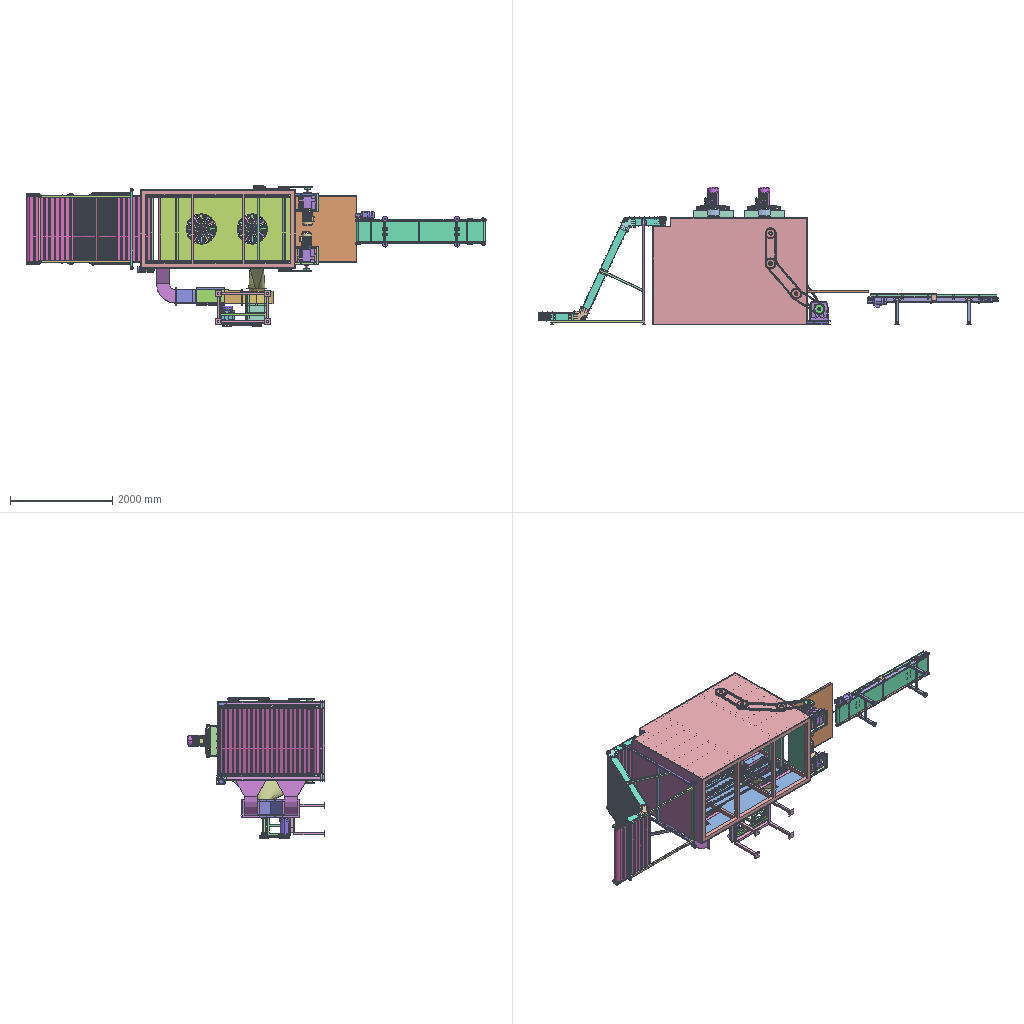Assembly | STEP file | 148 different items | 1898 placed | box 9018 x 2697 x 2745 mm
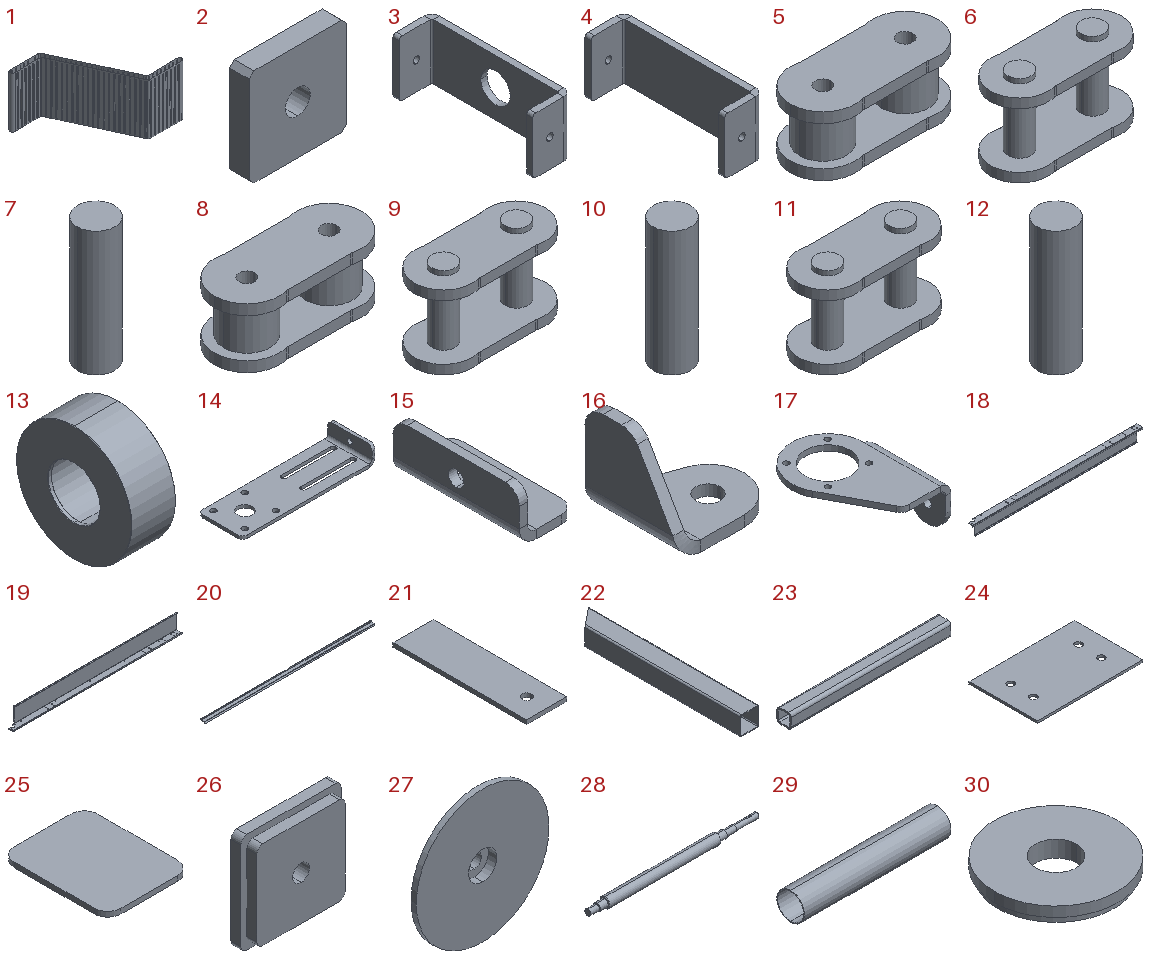Parts list (item | name | quantity | parent item | size | volume):
1 | Belt1-5^Produce dryer-Z conveyor | x1 | in Produce dryer-Z conveyor | 2487 x 2048 x 1290 mm | 28033863 mm3
2 | Bich chan tang chinh | x4 | in Produce dryer-Main support leg assembly | 40 x 8 x 40 mm | 12082 mm3
3 | Cang dai | x2 | in Produce dryer-Belt tensioner assembly | 25 x 90 x 36 mm | 17378 mm3
4 | Cang dai 2 | x2 | in Produce dryer-Belt tensioner assembly | 25 x 90 x 36 mm | 18513 mm3
5 | Chain 2-20A link 1 | x33 | in 链条2总成-00 | 56.75 x 25 x 23 mm | 16394 mm3
6 | Chain 2-20A link 2 | x33 | in 链条2总成-00 | 56.75 x 25 x 36 mm | 14459 mm3
7 | Chain 2-20A path | x1 | in 链条2总成-00 | 3 x 3 x 10 mm | 70.686 mm3
8 | Chain 3-20A link 1 | x56 | in 链条3总成-00 | 56.75 x 25 x 23 mm | 16394 mm3
9 | Chain 3-20A link 2 | x56 | in 链条3总成-00 | 56.75 x 25 x 36 mm | 14459 mm3
10 | Chain 3-20A path | x2 | in 链条3总成-00 | 3 x 3 x 10 mm | 70.686 mm3
11 | Chain 4-20A link 2 | x30 | in 链条4总成-00 | 56.75 x 25 x 36 mm | 14459 mm3
12 | Chain 4-20A path | x1 | in 链条4总成-00 | 3 x 3 x 10 mm | 70.686 mm3
13 | Con lan ty | x12 | in Roller assembly | 23 x 60 x 60 mm | 48906 mm3
14 | Flat conveyor mechanism-CN2500x400-101-101 | x2 | in 平输送机构-CN2500x400-101-100 | 270 x 90 x 36 mm | 137966 mm3
15 | Flat conveyor mechanism-CN2500x400-101-102 | x2 | in 平输送机构-CN2500x400-101-100 | 40 x 90 x 36 mm | 33488 mm3
16 | Flat conveyor mechanism-CN2500x400-102-101 | x1 | in Flat conveyor mechanism-CN2500x400-102-100 | 56 x 52 x 51 mm | 22223 mm3
17 | Flat conveyor mechanism-CN2500x400-102-102 | x1 | in Flat conveyor mechanism-CN2500x400-102-100 | 92 x 125 x 49 mm | 51756 mm3
18 | Flat conveyor mechanism-CN2500x400-103-101a | x1 | in Flat conveyor mechanism-assembly 2 | 2460 x 93 x 223 mm | 2426362 mm3
19 | Flat conveyor mechanism-CN2500x400-103-101b | x1 | in Flat conveyor mechanism-assembly 2 | 2460 x 100 x 223 mm | 2477714 mm3
20 | Flat conveyor mechanism-CN2500x400-104-101_DefaultSM-FLAT-PATTERN | x2 | in Flat conveyor mechanism-CN2500x400-104a-100, Flat conveyor mechanism-CN2500x400-104b-100 | 2450 x 58.268 x 35.821 mm | 594137 mm3
21 | Flat conveyor mechanism-CN2500x400-104-102 | x10 | in Flat conveyor mechanism-CN2500x400-104a-100, Flat conveyor mechanism-CN2500x400-104b-100 | 30 x 100 x 3 mm | 8885 mm3
22 | Flat conveyor mechanism-CN2500x400-105-101_Default<As machined> | x4 | in Flat conveyor mechanism-CN2500x400-105-100 | 50 x 450 x 50 mm | 160691 mm3
23 | Flat conveyor mechanism-CN2500x400-105-102_Default<As machined> | x2 | in Flat conveyor mechanism-CN2500x400-105-100 | 452 x 40 x 40 mm | 241728 mm3
24 | Flat conveyor mechanism-CN2500x400-105-103 | x4 | in Flat conveyor mechanism-CN2500x400-105-100 | 140 x 90 x 3 mm | 37037 mm3
25 | Flat conveyor mechanism-CN2500x400-105-104 | x4 | in Flat conveyor mechanism-CN2500x400-105-100 | 50 x 64 x 3 mm | 9435 mm3
26 | Flat conveyor mechanism-CN2500x400-105-105 | x4 | in Flat conveyor mechanism-CN2500x400-105-100 | 50 x 10 x 50 mm | 21535 mm3
27 | Flat conveyor mechanism-CN2500x400-105-106 | x4 | in 27 | 100 x 20 x 100 mm | 96687 mm3
28 | Flat conveyor mechanism-CN2500x400-107-101 | x1 | in Flat conveyor mechanism-CN2500x400-107-100 | 595.6 x 35 x 35 mm | 445688 mm3
29 | Flat conveyor mechanism-CN2500x400-107-102 | x2 | in Flat conveyor mechanism-CN2500x400-107-100, Flat conveyor mechanism-CN2500x400-108-100 | 400 x 75 x 75 mm | 183469 mm3
30 | Flat conveyor mechanism-CN2500x400-107-103 | x4 | in Flat conveyor mechanism-CN2500x400-107-100, Flat conveyor mechanism-CN2500x400-108-100 | 75 x 75 x 10 mm | 37435 mm3
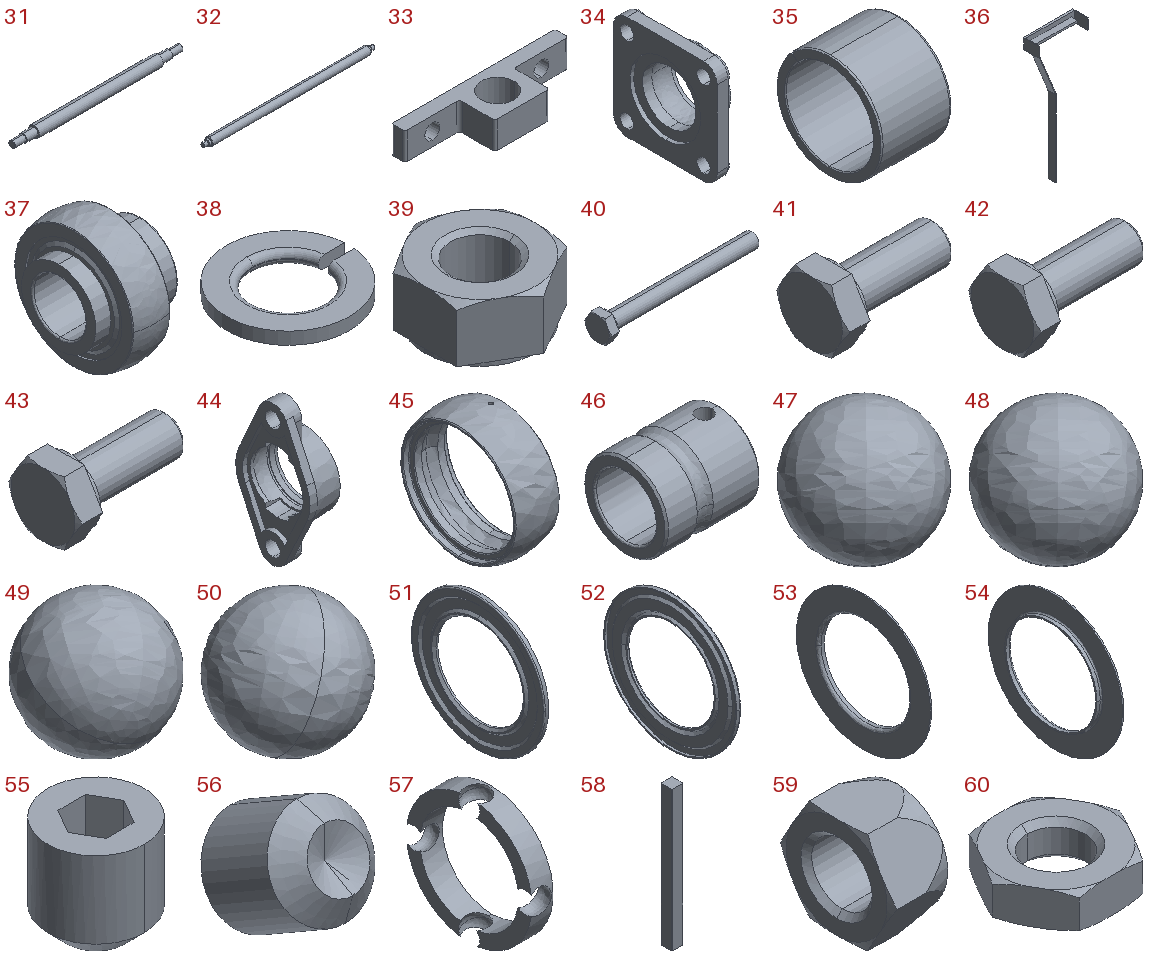31 | Flat conveyor mechanism-CN2500x400-108-101 | x1 | in Flat conveyor mechanism-CN2500x400-108-100 | 532 x 35 x 35 mm | 433255 mm3
32 | Flat conveyor mechanism-CN2500x400-111-101 | x3 | in Flat conveyor mechanism-CN2500x400-111-100 | 431 x 20 x 20 mm | 128796 mm3
33 | Flat conveyor mechanism-CN2500x400-111-102 | x6 | in Flat conveyor mechanism-CN2500x400-111-100 | 60 x 18 x 10 mm | 4223 mm3
34 | Flat conveyor mechanism-FY 504 U_VA228_fyva_Default | x2 | in Flat conveyor mechanism-FY 20 TF_VA228_Default | 29.5 x 86 x 86 mm | 59887 mm3
35 | Flat conveyor mechanism-PCM 101208 E.stp | x6 | in Flat conveyor mechanism-CN2500x400-111-100 | 8 x 12 x 12 mm | 274.832 mm3
36 | Flat conveyor mechanism-Part11 | x1 | in Flat conveyor mechanism-assembly 2 | 476 x 150 x 1294 mm | 1809742 mm3
37 | Flat conveyor mechanism-YAR 204-2FW_VA228_Default | x2 | in Flat conveyor mechanism-FY 20 TF_VA228_Default | 31 x 47 x 47 mm | 24116 mm3
38 | Flat conveyor mechanism-din_128_a12 | x12 | in 平输送机构-CN2500x400-101-100 | 21.067 x 21.1 x 2.1 mm | 456.756 mm3
39 | Flat conveyor mechanism-hex nut style 1 gradeab_din_Hexagon Nut ISO 4032 - M10 - W - N_Default | x4 | in 27 | 16 x 18.475 x 8.4 mm | 1357 mm3
40 | Flat conveyor mechanism-hex screw gradeab_din_DIN EN 24017 - M10 x 100-N_Default | x6 | in 27, 平输送机构-CN2500x400-101-100 | 106.4 x 18.475 x 16 mm | 9247 mm3
41 | Flat conveyor mechanism-hex screw gradeab_din_DIN EN 24017 - M10 x 25-N_Default | x2 | in Flat conveyor mechanism-assembly 2 | 31.4 x 18.475 x 16 mm | 3356 mm3
42 | Flat conveyor mechanism-hex screw gradeab_din_DIN EN 24017 - M6 x 16-N_Default | x16 | in Flat conveyor mechanism-assembly 2 | 20 x 11.547 x 10 mm | 791.21 mm3
43 | Flat conveyor mechanism-hex screw gradeab_din_DIN EN 24017 - M8 x 20-N_Default | x18 | in Flat conveyor mechanism-CN2500x400-102-100, Flat conveyor mechanism-assembly 2 | 25.3 x 15.011 x 13 mm | 1766 mm3
44 | Flat conveyor mechanism-inafag_ucfl204_62o9y6gnj3059x015y4y3bh4_01 | x2 | in Flat conveyor mechanism-inafag_ucfl204_62o9y6gnj3059x015y4y3bh4 | - | -
45 | Flat conveyor mechanism-inafag_ucfl204_62o9y6gnj3059x015y4y3bh4_02 | x2 | in Flat conveyor mechanism-inafag_ucfl204_62o9y6gnj3059x015y4y3bh4 | 17 x 47.603 x 47 mm | 6473 mm3
46 | Flat conveyor mechanism-inafag_ucfl204_62o9y6gnj3059x015y4y3bh4_03 | x2 | in Flat conveyor mechanism-inafag_ucfl204_62o9y6gnj3059x015y4y3bh4 | 31 x 27.56 x 27.56 mm | 8243 mm3
47 | Flat conveyor mechanism-inafag_ucfl204_62o9y6gnj3059x015y4y3bh4_04 | x2 | in Flat conveyor mechanism-inafag_ucfl204_62o9y6gnj3059x015y4y3bh4 | 7.94 x 7.94 x 7.94 mm | 262.089 mm3
48 | Flat conveyor mechanism-inafag_ucfl204_62o9y6gnj3059x015y4y3bh4_05 | x2 | in Flat conveyor mechanism-inafag_ucfl204_62o9y6gnj3059x015y4y3bh4 | 7.94 x 7.94 x 7.94 mm | 262.089 mm3
49 | Flat conveyor mechanism-inafag_ucfl204_62o9y6gnj3059x015y4y3bh4_06 | x2 | in Flat conveyor mechanism-inafag_ucfl204_62o9y6gnj3059x015y4y3bh4 | 7.94 x 7.94 x 7.94 mm | 262.089 mm3
50 | Flat conveyor mechanism-inafag_ucfl204_62o9y6gnj3059x015y4y3bh4_07 | x2 | in Flat conveyor mechanism-inafag_ucfl204_62o9y6gnj3059x015y4y3bh4 | 7.94 x 7.94 x 7.94 mm | 262.089 mm3
51 | Flat conveyor mechanism-inafag_ucfl204_62o9y6gnj3059x015y4y3bh4_08 | x2 | in Flat conveyor mechanism-inafag_ucfl204_62o9y6gnj3059x015y4y3bh4 | 1.397 x 42 x 42 mm | 599.425 mm3
52 | Flat conveyor mechanism-inafag_ucfl204_62o9y6gnj3059x015y4y3bh4_09 | x2 | in Flat conveyor mechanism-inafag_ucfl204_62o9y6gnj3059x015y4y3bh4 | 1.397 x 42 x 42 mm | 599.533 mm3
53 | Flat conveyor mechanism-inafag_ucfl204_62o9y6gnj3059x015y4y3bh4_10 | x2 | in Flat conveyor mechanism-inafag_ucfl204_62o9y6gnj3059x015y4y3bh4 | 1.812 x 41.16 x 41.16 mm | 343.087 mm3
54 | Flat conveyor mechanism-inafag_ucfl204_62o9y6gnj3059x015y4y3bh4_11 | x2 | in Flat conveyor mechanism-inafag_ucfl204_62o9y6gnj3059x015y4y3bh4 | 1.812 x 41.16 x 41.16 mm | 343.35 mm3
55 | Flat conveyor mechanism-inafag_ucfl204_62o9y6gnj3059x015y4y3bh4_12 | x2 | in Flat conveyor mechanism-inafag_ucfl204_62o9y6gnj3059x015y4y3bh4 | 6 x 6 x 6 mm | 135.214 mm3
56 | Flat conveyor mechanism-inafag_ucfl204_62o9y6gnj3059x015y4y3bh4_13 | x2 | in Flat conveyor mechanism-inafag_ucfl204_62o9y6gnj3059x015y4y3bh4 | 6 x 7.571 x 7.571 mm | 135.214 mm3
57 | Flat conveyor mechanism-inafag_ucfl204_62o9y6gnj3059x015y4y3bh4_14 | x2 | in Flat conveyor mechanism-inafag_ucfl204_62o9y6gnj3059x015y4y3bh4 | - | 2155 mm3
58 | Flat conveyor mechanism-key 6x6x70 | x1 | in Flat conveyor mechanism-assembly 2 | 6 x 6 x 75 mm | 2686 mm3
59 | Flat conveyor mechanism-nut_gb_t_6185_1_m6 | x16 | in Flat conveyor mechanism-assembly 2 | 6 x 11.547 x 10 mm | 336.581 mm3
60 | Flat conveyor mechanism-nut_iso_4035_-_d_m10_-_05 | x32 | in 平输送机构-CN2500x400-101-100 | 18.475 x 16 x 5 mm | 809.954 mm3
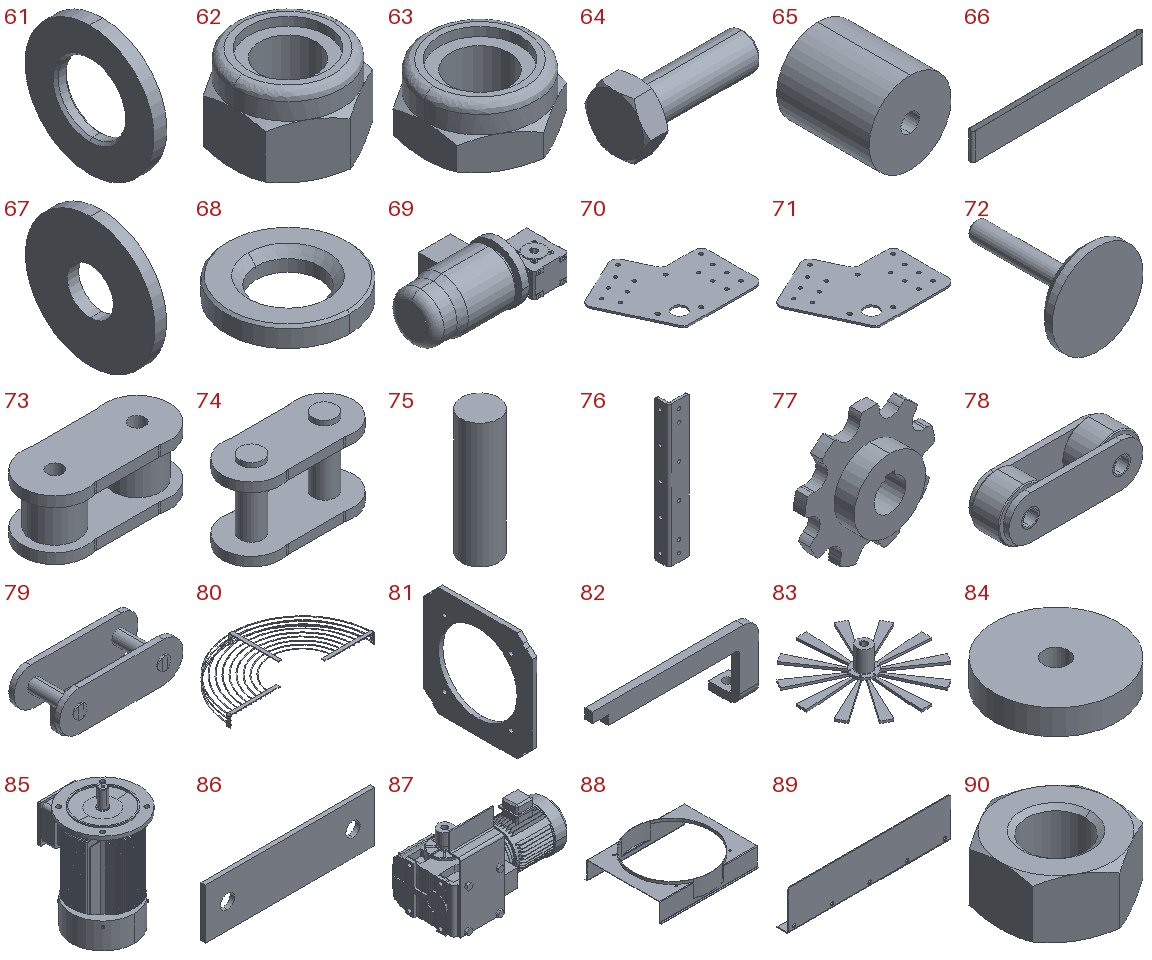61 | Flat conveyor mechanism-plain washer hardened grade a_din_Washer DIN 125 - A 10.5 - 300HV_Default | x4 | in Flat conveyor mechanism-assembly 2 | 2 x 20 x 20 mm | 449.726 mm3
62 | Flat conveyor mechanism-prevailing torque nut style 1 insert_din_DIN EN ISO 7040 - M8 - N_Default | x16 | in Flat conveyor mechanism-assembly 2 | 13 x 15.011 x 9.5 mm | 952.721 mm3
63 | Flat conveyor mechanism-prevailing torque nut thin insert_din_DIN EN ISO 10511 - M10 - N_Default | x2 | in Flat conveyor mechanism-assembly 2 | 16 x 18.475 x 8.56 mm | 1235 mm3
64 | Flat conveyor mechanism-screw_gb_t_6563_m10x30 | x20 | in 平输送机构-CN2500x400-101-100 | 36.4 x 18.475 x 16 mm | 3756 mm3
65 | Flat conveyor mechanism-silenbloc 40x45xm8 | x1 | in Flat conveyor mechanism-CN2500x400-102-100 | 40 x 45 x 40 mm | 54907 mm3
66 | Flat conveyor mechanism-strip | x1 | in Flat conveyor mechanism-assembly 2 | 2534 x 103.36 x 400 mm | 5769946 mm3
67 | Flat conveyor mechanism-washer_gb_t_96_1_6 | x12 | in Flat conveyor mechanism-assembly 2 | 1.6 x 18 x 18 mm | 355.679 mm3
68 | Flat conveyor mechanism-washer_iso_7416-12 | x40 | in 平输送机构-CN2500x400-101-100 | 25 x 25 x 4 mm | 1366 mm3
69 | Flat conveyor mechanism-worm gear reducer_mu40-base-10-b3 | x1 | in Flat conveyor mechanism-assembly 2 | 361 x 200 x 160 mm | 5383182 mm3
70 | Ga bi suong | x2 | in Produce dryer-Belt tensioner corner assembly | 306.397 x 266.767 x 5 mm | 273503 mm3
71 | Ga bi suong 2 | x2 | in Produce dryer-Corner belt tensioner assembly 2 | 306.397 x 266.767 x 5 mm | 273503 mm3
72 | Main support leg M12 for conveyor | x4 | in Produce dryer-Main support leg assembly | 60 x 80 x 60 mm | 33948 mm3
73 | Motor output chain-06B link 1 | x24 | in 电机输出链条-00 | 56.75 x 25 x 23 mm | 16394 mm3
74 | Motor output chain-06B link 2 | x24 | in 电机输出链条-00 | 56.75 x 25 x 36 mm | 14459 mm3
75 | Motor output chain-motor drive chain path 1 | x1 | in 电机输出链条-00 | 3 x 3 x 10 mm | 70.686 mm3
76 | Part 1 cang dai | x4 | in Produce dryer-Belt tensioner assembly | 36 x 25 x 250 mm | 54427 mm3
77 | Produce dryer 9-tooth 40 bore with keyway total width 40 C216AL sprocket | x20 | in Produce dryer single mesh belt assembly, Produce dryer single mesh belt assembly C | 163.79 x 40 x 161.93 mm | 358621 mm3
78 | Produce dryer C216AL inner link | x470 | in Produce dryer single mesh belt assembly, Produce dryer single mesh belt assembly C | - | -
79 | Produce dryer C216AL outer link | x470 | in Produce dryer single mesh belt assembly, Produce dryer single mesh belt assembly C | - | -
80 | Produce dryer HY-40-M-021 | x4 | in Produce dryer HY-40-M-700 | 645 x 322.5 x 50 mm | 90254 mm3
81 | Produce dryer HY-40-M-701 | x2 | in Produce dryer HY-40-M-710 | 10 x 250 x 250 mm | 341607 mm3
82 | Produce dryer HY-40-M-702 | x8 | in Produce dryer HY-40-M-710 | 215 x 40 x 90 mm | 72091 mm3
83 | Produce dryer HY-40-M-809 | x2 | in Produce dryer HY-40-M-700 | 550 x 550 x 113 mm | 1036820 mm3
84 | Produce dryer HY-40-M-bushing clamp plate | x2 | in Produce dryer HY-40-M-700 | 49 x 49 x 10 mm | 18072 mm3
85 | Produce dryer YE3-100L-4-B5_YE4-100L-2 | x2 | in Produce dryer HY-40-M-700 | 250 x 295 x 435 mm | 12374001 mm3
86 | Produce dryer bearing housing pad plate | x10 | in Produce dryer mesh belt assembly Type A, Produce dryer mesh belt assembly Type B, Produce dryer mesh belt assembly Type C | 185 x 5 x 55 mm | 48988 mm3
87 | Produce dryer conveyor belt NSNS47 reducer_NS 67 | x1 | in Produce dryer-Z conveyor | 331.6 x 173.674 x 227.5 mm | 3816631 mm3
88 | Produce dryer cooling section-HY-40-M-601 | x2 | in Produce dryer cooling section-HY-40-M-cover assembly | 786 x 630 x 168 mm | 1349163 mm3
89 | Produce dryer cooling section-HY-40-M-602 | x4 | in Produce dryer cooling section-HY-40-M-cover assembly | 584 x 40 x 142 mm | 308453 mm3
90 | Produce dryer cooling section-hex nut style 1_am_B18.2.4.1M - Hex nut, Style 1, M10 x 1.5 | x8 | in Produce dryer cooling section-HY-40-M-cover assembly | 16 x 18.475 x 8.4 mm | 1365 mm3
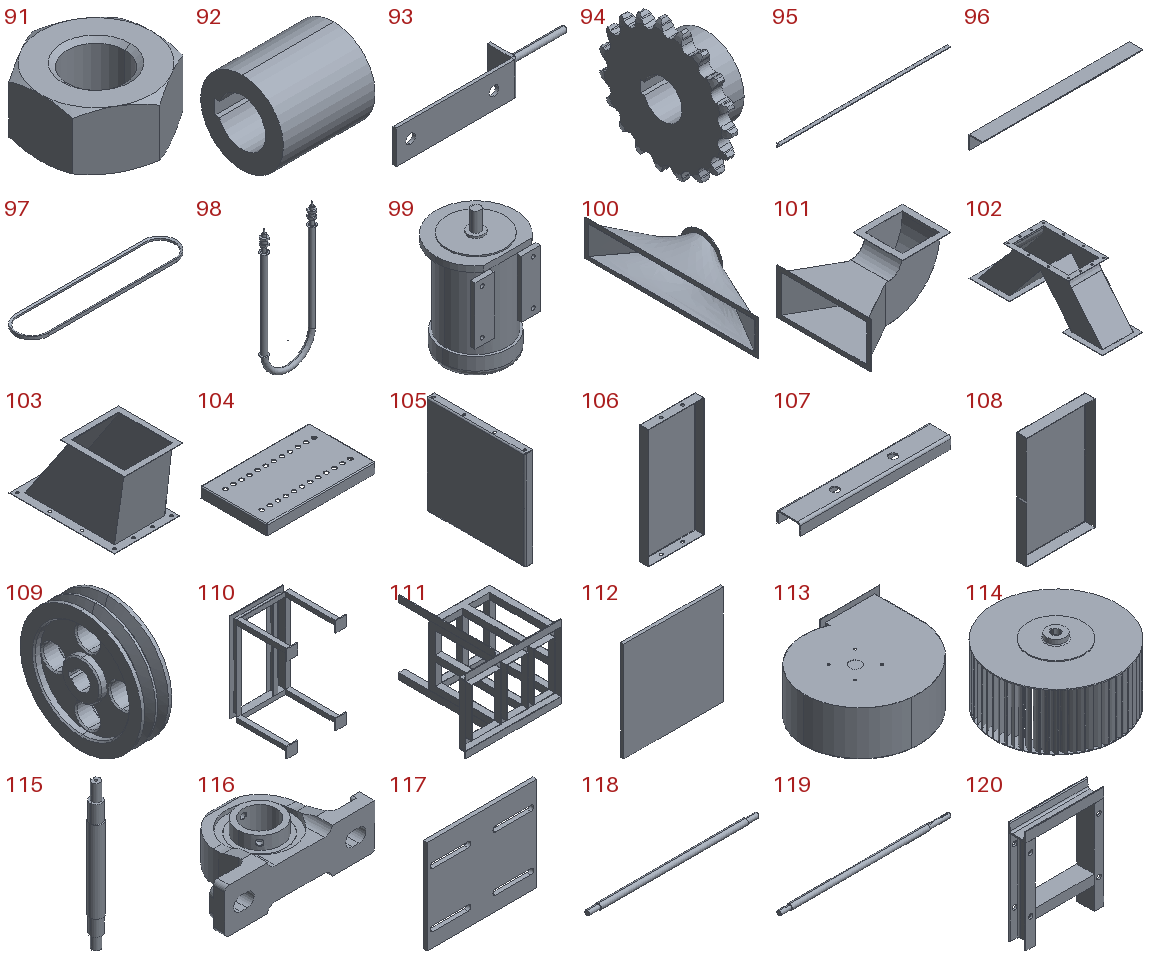91 | Produce dryer cooling section-hex nut style 1_am_B18.2.4.1M - Hex nut, Style 1, M8 x 1.25 | x20 | in Produce dryer cooling section-HY-40-M-cover assembly | 13 x 15.011 x 6.8 mm | 737.453 mm3
92 | Produce dryer double-row sprocket | x5 | in Produce dryer 19-tooth 40 bore with keyway 20A double-row driven sprocket | 78 x 70 x 70 mm | 199069 mm3
93 | Produce dryer driven tensioner plate | x10 | in Produce dryer mesh belt assembly Type A, Produce dryer mesh belt assembly Type B, Produce dryer mesh belt assembly Type C | 306.4 x 45 x 55 mm | 72873 mm3
94 | Produce dryer driving sprocket-1_20A | x2 | in 果蔬烘干机-100 (2) | 67 x 205.935 x 206.617 mm | 832026 mm3
95 | Produce dryer frame-10_Default<As Machined> | x8 | in 果蔬烘干机-100 (2) | 1850 x 40 x 40 mm | 702264 mm3
96 | Produce dryer frame-6_Default<As Machined> | x20 | in 果蔬烘干机-100 (2) | 940 x 80 x 80 mm | 709111 mm3
97 | Produce dryer line heating fan-BELT-B | x2 | in Produce dryer line heating fan-SIROCCOFAN-3KW-000 | 896 x 182 x 17 mm | 281453 mm3
98 | Produce dryer line heating fan-HEATER-U | x12 | in Produce dryer line heating fan-OVEN-450 | 210 x 30 x 509.5 mm | 300889 mm3
99 | Produce dryer line heating fan-MOYOT-Y100L2-4(3KW) | x1 | in Produce dryer line heating fan-SIROCCOFAN-3KW-000 | 250 x 230 x 390 mm | 10532784 mm3
100 | Produce dryer line heating fan-OVEN-401 | x1 | in Produce dryer line heating fan-OVEN-000 | 403.502 x 1600 x 395 mm | 2039591 mm3
101 | Produce dryer line heating fan-OVEN-402 | x2 | in Produce dryer line heating fan-OVEN-420 | 721.5 x 660 x 410 mm | 1592936 mm3
102 | Produce dryer line heating fan-OVEN-422 | x1 | in Produce dryer line heating fan-OVEN-420 | 340 x 1130 x 403 mm | 1800056 mm3
103 | Produce dryer line heating fan-OVEN-445 | x1 | in Produce dryer line heating fan-OVEN-450 | 345.008 x 567.391 x 339.5 mm | 1076631 mm3
104 | Produce dryer line heating fan-OVEN-451 | x1 | in Produce dryer line heating fan-OVEN-450 | 540 x 330 x 51 mm | 750332 mm3
105 | Produce dryer line heating fan-OVEN-452 | x1 | in Produce dryer line heating fan-OVEN-450 | 42 x 550 x 550 mm | 763414 mm3
106 | Produce dryer line heating fan-OVEN-453 | x1 | in Produce dryer line heating fan-OVEN-450 | 260 x 42 x 550 mm | 408426 mm3
107 | Produce dryer line heating fan-OVEN-454 | x2 | in Produce dryer line heating fan-OVEN-450 | 260 x 40 x 20 mm | 37565 mm3
108 | Produce dryer line heating fan-OVEN-455 | x1 | in Produce dryer line heating fan-OVEN-450 | 340 x 52 x 550 mm | 543570 mm3
109 | Produce dryer line heating fan-PULLY-B-2-150 | x2 | in Produce dryer line heating fan-SIROCCOFAN-3KW-000 | 45 x 180 x 180 mm | 597383 mm3
110 | Produce dryer line heating fan-SIROCCOFAN-3KW-001 | x1 | in Produce dryer line heating fan-SIROCCOFAN-3KW-000 | 670 x 680 x 1070 mm | 10335392 mm3
111 | Produce dryer line heating fan-SIROCCOFAN-3KW-101 | x1 | in Produce dryer line heating fan-SIROCCOFAN-3KW-100 | 600 x 640 x 460 mm | 2910476 mm3
112 | Produce dryer line heating fan-SIROCCOFAN-3KW-102 | x1 | in Produce dryer line heating fan-SIROCCOFAN-3KW-100 | 380 x 12 x 380 mm | 1732800 mm3
113 | Produce dryer line heating fan-SIROCCOFAN-3KW-COVER | x1 | in Produce dryer line heating fan-SIROCCOFAN-3KW-100 | 718 x 612.214 x 321 mm | 2543268 mm3
114 | Produce dryer line heating fan-SIROCCOFAN-3KW-ROLLER | x1 | in Produce dryer line heating fan-SIROCCOFAN-3KW-100 | 400 x 400 x 205 mm | 1898819 mm3
115 | Produce dryer line heating fan-SIROCCOFAN-3KW-SHAFT | x1 | in Produce dryer line heating fan-SIROCCOFAN-3KW-000 | 45 x 45 x 498 mm | 647195 mm3
116 | Produce dryer line heating fan-UCP208_PDR40 | x2 | in Produce dryer line heating fan-SIROCCOFAN-3KW-100 | 184 x 108 x 57.2 mm | 354732 mm3
117 | Produce dryer line heating fan-motor base | x1 | in Produce dryer line heating fan-SIROCCOFAN-3KW-000 | 280 x 10 x 240 mm | 615442 mm3
118 | Produce dryer mesh belt driven shaft | x5 | in Produce dryer mesh belt assembly Type A, Produce dryer mesh belt assembly Type B, Produce dryer mesh belt assembly Type C | 1461 x 50 x 50 mm | 2725239 mm3
119 | Produce dryer mesh belt driving shaft | x5 | in Produce dryer mesh belt assembly Type A, Produce dryer mesh belt assembly Type B, Produce dryer mesh belt assembly Type C | 1562 x 50 x 50 mm | 2850228 mm3
120 | Produce dryer motor mount_Default<As Machined> | x2 | in 果蔬烘干机-110 | 353 x 80 x 466.5 mm | 1481860 mm3
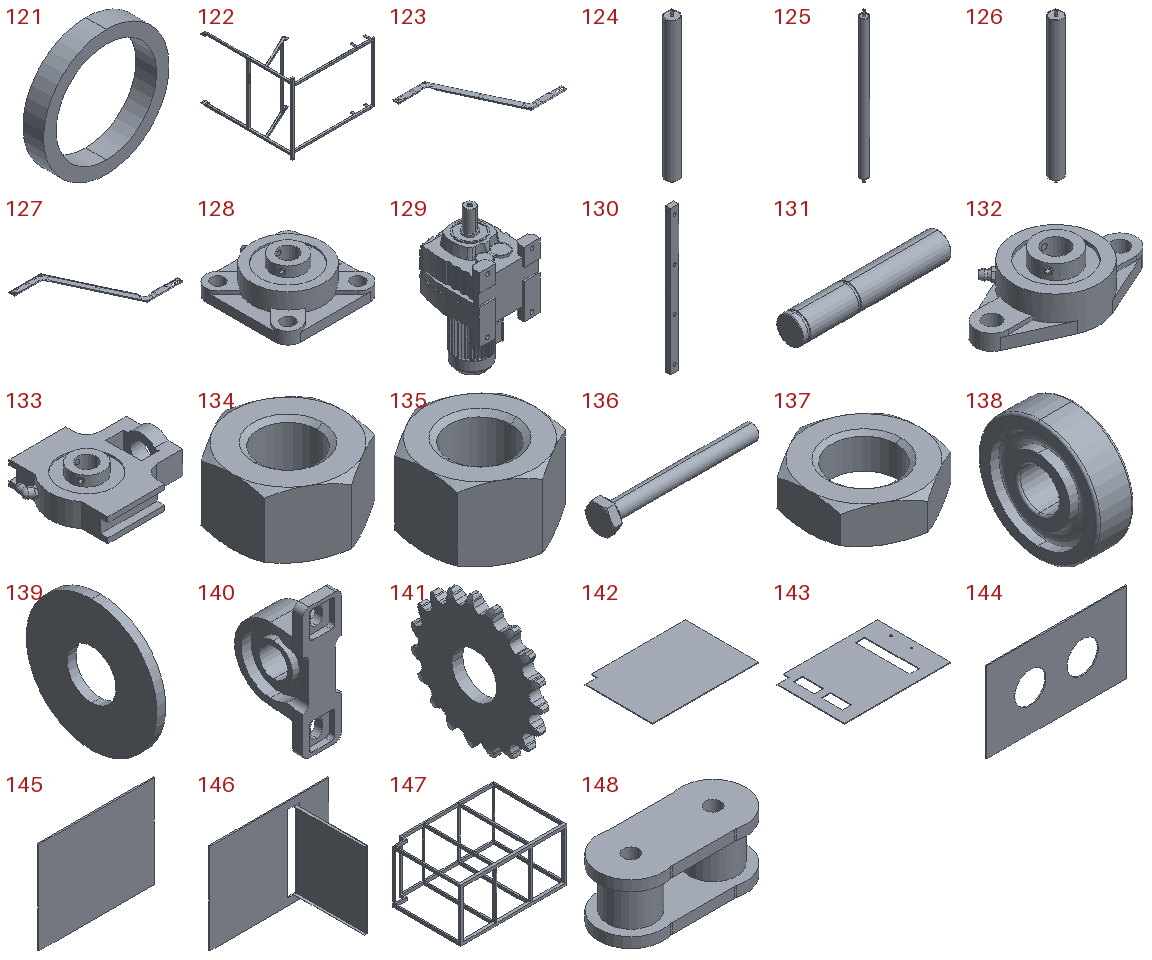121 | Produce dryer shaft collar | x20 | in Produce dryer mesh belt assembly Type A, Produce dryer mesh belt assembly Type B, Produce dryer mesh belt assembly Type C | 50 x 8.25 x 50 mm | 5832 mm3
122 | Produce dryer-Conveyor frame_Default<As Machined> | x1 | in Produce dryer-Z conveyor | 1870 x 2016 x 1574 mm | 3631484 mm3
123 | Produce dryer-Conveyor side plate 1 | x1 | in Produce dryer-Z conveyor | 2506 x 2006 x 25 mm | 2012083 mm3
124 | Produce dryer-Driven part | x1 | in Produce dryer-Z conveyor | 124 x 124 x 1393 mm | 2869767 mm3
125 | Produce dryer-Driven part 2 | x2 | in Produce dryer-Z conveyor | 73 x 73 x 1397 mm | 1653987 mm3
126 | Produce dryer-Driving part | x1 | in Produce dryer-Z conveyor | 124 x 124 x 1402 mm | 2870490 mm3
127 | Produce dryer-Mirror conveyor side plate 1 | x1 | in Produce dryer-Z conveyor | 2506 x 2006 x 25 mm | 2012083 mm3
128 | Produce dryer-ucf203 | x2 | in Produce dryer-Z conveyor | 86 x 86 x 33.3 mm | 92180 mm3
129 | R97-216.28-2.2-M1-0° R97 helical gear reducer | x2 | in 果蔬烘干机-100 (2) | 348 x 368 x 773.5 mm | 40162039 mm3
130 | Rãnh trượt | x4 | in Produce dryer-Belt tensioner assembly | 11.5 x 7 x 200 mm | 15712 mm3
131 | Truc con lan | x12 | in Roller assembly | 56 x 10 x 10 mm | 4376 mm3
132 | UCFL203 | x4 | in Produce dryer-Belt tensioner corner assembly, Produce dryer-Corner belt tensioner assembly 2 | 113 x 60 x 33.3 mm | 69003 mm3
133 | UCT203 | x2 | in Produce dryer-Belt tensioner assembly | 99.208 x 89 x 34.3 mm | 116235 mm3
134 | hex nut gradec_iso_ISO - 4034 - M10 - N | x24 | in Produce dryer-Belt tensioner corner assembly, Produce dryer-Corner belt tensioner assembly 2 | 16 x 18.475 x 9.5 mm | 1547 mm3
135 | hex nut gradec_iso_ISO - 4034 - M12 - N | x8 | in Produce dryer-Main support leg assembly | 18 x 20.785 x 12.2 mm | 2394 mm3
136 | hex structural bolt gradec short_iso_ISO 7412 - M16 x 150 --- 38-WN | x2 | in Produce dryer-Belt tensioner assembly | 160 x 31.177 x 27 mm | 36375 mm3
137 | hex thin nut chamfered gradeab_iso_ISO - 4035 - M16 - N | x4 | in Produce dryer-Belt tensioner assembly | 24 x 27.713 x 8 mm | 2696 mm3
138 | radial ball bearing_68_skf_SKF - 6200 - 8,SI,NC,8_68 | x24 | in Roller assembly | 9 x 30 x 30 mm | 4761 mm3
139 | 平输送机构-625058 | x2 | in Flat conveyor mechanism-CN2500x400-102-100 | 1.5 x 22 x 22 mm | 490.015 mm3
140 | 果蔬烘干机-208 轴承座 | x20 | in Produce dryer mesh belt assembly Type A, Produce dryer mesh belt assembly Type B, Produce dryer mesh belt assembly Type C | 57.2 x 100 x 184 mm | 317454 mm3
141 | 果蔬烘干机从动链轮-19齿_20A | x10 | in Produce dryer 19-tooth 40 bore with keyway 20A double-row driven sprocket | 17 x 205.935 x 206.617 mm | 397134 mm3
142 | 果蔬烘干机框架-103 | x1 | in 果蔬烘干机-100 (2) | 3000 x 2080 x 20 mm | 123712000 mm3
143 | 果蔬烘干机框架-104 | x1 | in 果蔬烘干机-100 (2) | 3000 x 2080 x 20 mm | 109217649 mm3
144 | 果蔬烘干机框架-105 | x1 | in 果蔬烘干机-100 (2) | 2660 x 20 x 1540 mm | 70618266 mm3
145 | 果蔬烘干机框架-106 | x1 | in 果蔬烘干机-100 (2) | 1920 x 20 x 1540 mm | 59136000 mm3
146 | 果蔬烘干机框架-107 | x1 | in 果蔬烘干机-100 (2) | 2020 x 1220 x 1540 mm | 60915530 mm3
147 | 果蔬烘干机框架-111 | x1 | in 果蔬烘干机-110 | 3000 x 2080 x 1500 mm | 144224000 mm3
148 | 链条4-20A链节1 | x30 | in 链条4总成-00 | 56.75 x 25 x 23 mm | 16394 mm3